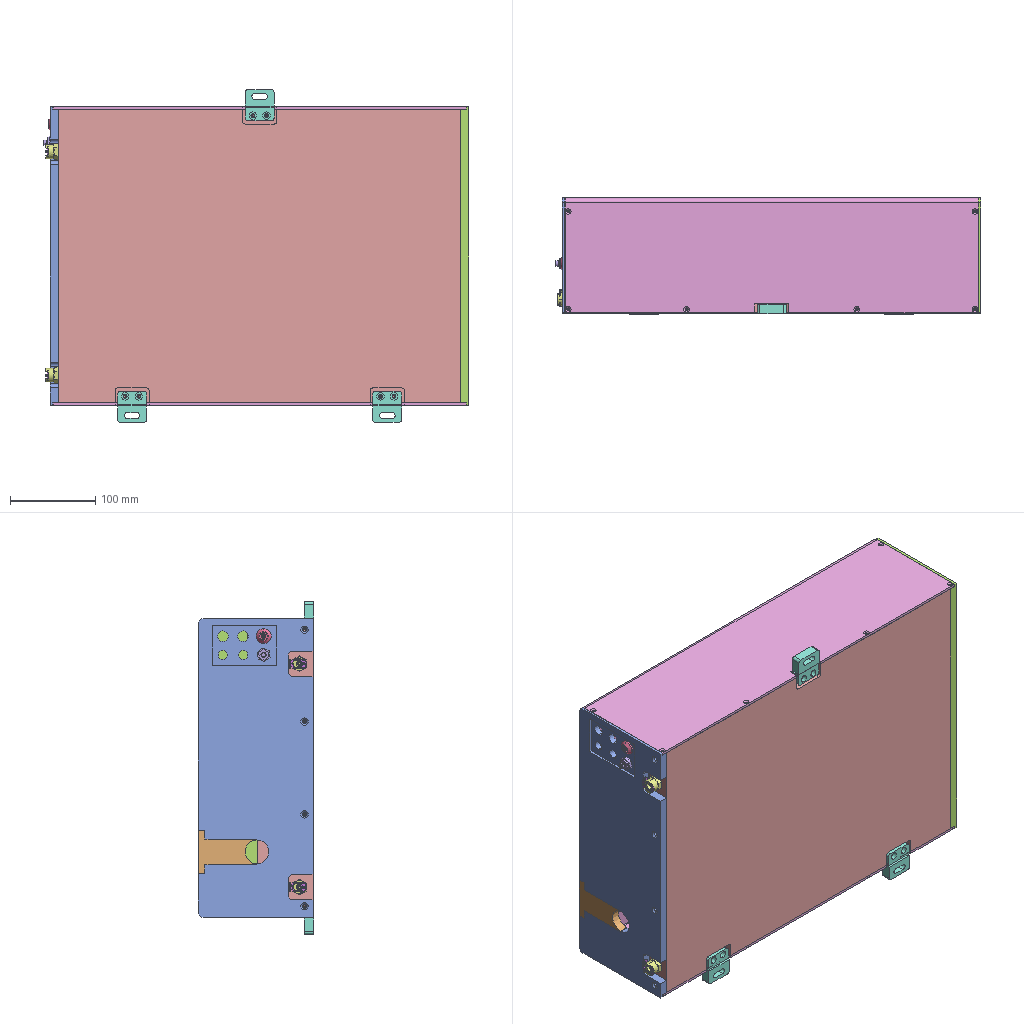Assembly | SolidWorks | 13 different items | 18 placed | box 501 x 136 x 391 mm
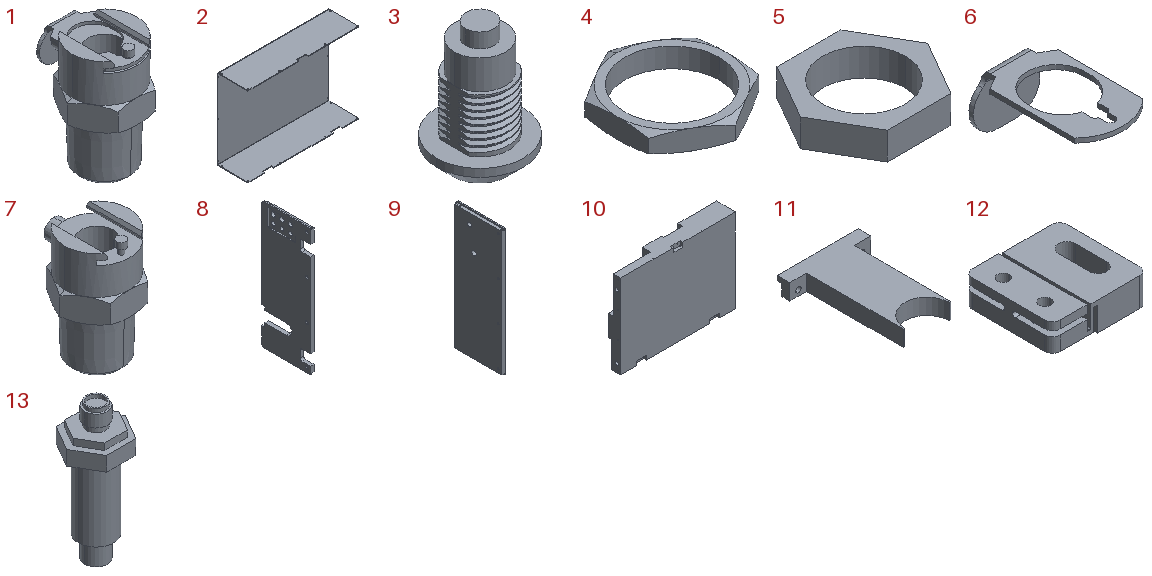Parts list (item | name | quantity | parent item | size | volume | features):
1 | (subassembly) | x2 | - | 18.478 x 19.431 x 28.448 mm | 3928 mm3 | -
2 | - | x1 | - | 485.5 x 135 x 351 mm | 883861 mm3 | features HoleWzd 3, Cut 2, Fillet 2, ICE 2, Extrusion 1
3 | - | x1 | - | 17.8 x 17.8 x 25 mm | 2223 mm3 | features ICE 7, Chamfer 1, Extrusion 1, Fillet 1, SweepThread 1
4 | - | x1 | - | 14 x 16.166 x 2.5 mm | 137.79 mm3 | features Extrusion 1, RevCut 1
5 | - | x1 | - | 13.856 x 12 x 3 mm | 183.271 mm3 | features Extrusion 1, HoleWzd 1
6 | - | x2 | in 1 | 10.922 x 19.304 x 8.89 mm | 127.415 mm3 | features BaseBody 1
7 | - | x2 | in 1 | 18.478 x 18.72 x 28.448 mm | 3801 mm3 | features BaseBody 1
8 | - | x1 | - | 10 x 135 x 351 mm | 402993 mm3 | features Cut 47, HoleWzd 41, MoveFace 39, ICE 28, Fillet 19, DelFace 17, MirrorPattern 3, SweepCut 2, Extrusion 1
9 | - | x1 | - | 10 x 135 x 351 mm | 457423 mm3 | features Cut 44, HoleWzd 41, MoveFace 38, ICE 28, DelFace 17, Fillet 17, MirrorPattern 3, SweepCut 2, Extrusion 1
10 | - | x1 | - | 472 x 78 x 345 mm | 7845697 mm3 | features Cut 44, HoleWzd 43, MoveFace 39, ICE 30, DelFace 19, Fillet 18, MirrorPattern 5, SweepCut 2, Extrusion 1
11 | - | x1 | - | 51 x 69 x 10 mm | 18117 mm3 | features MoveFace 4, ICE 3, Cut 2, HoleWzd 2, Extrusion 1, MirrorPattern 1
12 | - | x3 | - | 36.5 x 34 x 11.5 mm | 9581 mm3 | features ICE 13, MoveFace 5, Fillet 3, DelFace 2, Extrusion 1, PLine 1
13 | - | x1 | - | 16.166 x 14 x 37.6 mm | 2584 mm3 | features ICE 5, Extrusion 1
Mates (type | each side: item.copy, entity, surface, feature):
Coincident | 10.1 face plane Cut-Extrude56 | 8.1 face plane Cut-Extrude19
Coincident | 10.1 face plane Cut-Extrude56 | 9.1 face plane Cut-Extrude19
Coincident | 8.1 face plane Boss-Extrude17 | 9.1 face plane Boss-Extrude16 | 2 times
Coincident | 10.1 face plane Cut-Extrude56 | 2.1 face plane Boss-Extrude1
Coincident | 10.1 face plane Cut-Extrude10 | 2.1 face plane Boss-Extrude1
Width | 8.1 face plane Cut-Extrude19 | 9.1 face plane Cut-Extrude19 | 2.1 face plane Boss-Extrude1 | 2.1 face plane Boss-Extrude1
Coincident | 10.1 face plane Cut-Extrude57 | 12.1 face plane Boss-Extrude3
Concentric | 10.1 face cylinder M4 Tapped Hole18 | 12.1 face cylinder Cut-Extrude5 | 2 times
Coincident | 10.1 face plane Cut-Extrude57 | 12.2 face plane Boss-Extrude3
Concentric | 10.1 face cylinder M4 Tapped Hole18 | 12.2 face cylinder Cut-Extrude5 | 2 times
Coincident | 10.1 face plane Cut-Extrude57 | 12.3 face plane Boss-Extrude3
Concentric | 10.1 face cylinder M4 Tapped Hole18 | 12.3 face cylinder Cut-Extrude5 | 2 times
Coincident | 8.1 face plane Boss-Extrude17 | 11.1 face plane Boss-Extrude1
Concentric | 8.1 face cylinder Cut-Extrude25 | 11.1 face cylinder Boss-Extrude1
Coincident | 8.1 face plane Cut-Extrude26 | 11.1 face plane Boss-Extrude1
Coincident | 8.1 face plane Cut-Extrude59 | 3.1 face plane Boss-Extrude1
Concentric | 8.1 face cylinder Cut-Extrude60 | 3.1 face cylinder Boss-Extrude3
Concentric | 3.1 face cylinder Boss-Extrude3 | 4.1 face cylinder Boss-Extrude1
Coincident | 8.1 face plane Cut-Extrude19 | 4.1 face plane Boss-Extrude1
Concentric | 8.1 face cylinder Cut-Extrude60 | 13.1 face cylinder Boss-Extrude5
Coincident | 8.1 face plane Cut-Extrude59 | 13.1 face plane Boss-Extrude1
Concentric | 13.1 face cylinder Boss-Extrude6 | 5.1 face cylinder M10x1.0 Tapped Hole1
Coincident | 8.1 face plane Cut-Extrude19 | 5.1 face plane Boss-Extrude1
Coincident | 10.1 face plane Cut-Extrude56 | 7.1 face plane Input 1
Concentric | 10.1 face cylinder Cut-Sweep1 | 7.2 face cone Input 1
Coincident | 10.1 face plane Cut-Extrude56 | 7.2 face plane Input 1
Coincident | 8.1 face plane Boss-Extrude11 | 2.1 face plane Boss-Extrude2
Coincident | 8.1 face plane Boss-Extrude20 | 2.1 face plane Boss-Extrude3
Concentric | 10.1 face cylinder Cut-Sweep3 | 7.1 face cone Input 1